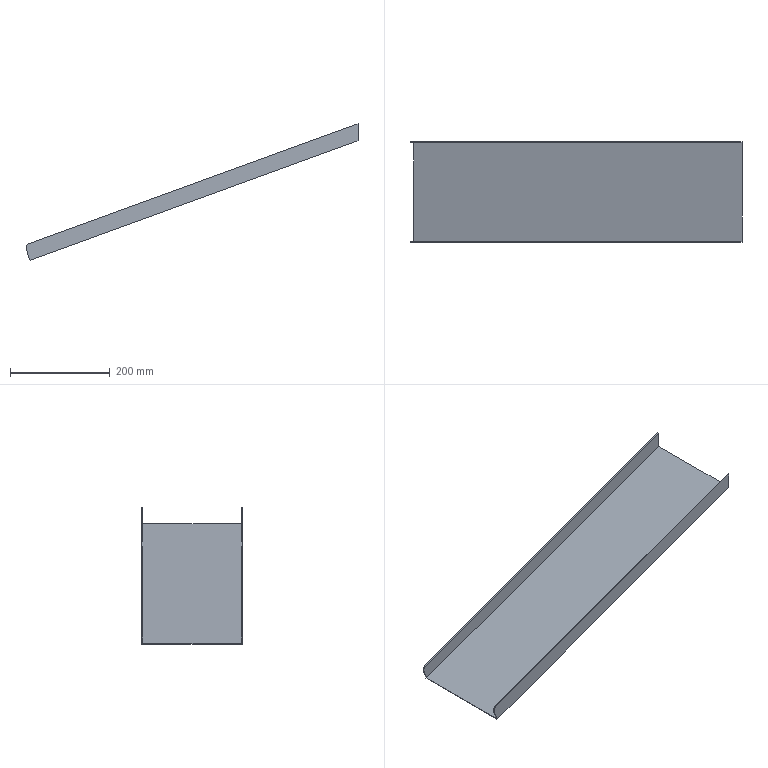Part | NX | features HB 2 | 1 solid | 12 faces | box 664.956 x 201 x 273.12 mm | volume 365672 mm3 | plane 10 | cylinder 2 | commonest cylinder face diameters 20 x2
STEP:
#1=CARTESIAN_POINT('',(3932.421,98.421,-251.344));
#2=VERTEX_POINT('',#1);
#3=CARTESIAN_POINT('',(3274.909,98.421,-490.659));
#4=VERTEX_POINT('',#3);
#5=CARTESIAN_POINT('',(3821.81,98.421,-291.603));
#6=DIRECTION('',(-0.9397,0.,-0.342));
#7=VECTOR('',#6,1000.);
#8=LINE('',#5,#7);
#9=EDGE_CURVE('',#2,#4,#8,.T.);
#10=ORIENTED_EDGE('',*,*,#9,.F.);
#11=CARTESIAN_POINT('',(3932.421,98.421,-219.418));
#12=VERTEX_POINT('',#11);
#13=CARTESIAN_POINT('',(3932.421,98.421,-291.603));
#14=DIRECTION('',(0.,0.,1.));
#15=VECTOR('',#14,1000.);
#16=LINE('',#13,#15);
#17=EDGE_CURVE('',#2,#12,#16,.T.);
#18=ORIENTED_EDGE('',*,*,#17,.T.);
#19=CARTESIAN_POINT('',(3274.045,98.421,-459.048));
#20=VERTEX_POINT('',#19);
#21=CARTESIAN_POINT('',(3811.549,98.421,-263.412));
#22=DIRECTION('',(0.9397,0.,0.342));
#23=VECTOR('',#22,1000.);
#24=LINE('',#21,#23);
#25=EDGE_CURVE('',#20,#12,#24,.T.);
#26=ORIENTED_EDGE('',*,*,#25,.F.);
#27=CARTESIAN_POINT('',(3268.068,98.421,-471.865));
#28=VERTEX_POINT('',#27);
#29=CARTESIAN_POINT('',(3277.465,98.421,-468.445));
#30=DIRECTION('',(0.,1.,0.));
#31=DIRECTION('',(0.,0.,1.));
#32=AXIS2_PLACEMENT_3D('',#29,#30,#31);
#33=CIRCLE('',#32,10.);
#34=EDGE_CURVE('',#28,#20,#33,.T.);
#35=ORIENTED_EDGE('',*,*,#34,.F.);
#36=CARTESIAN_POINT('',(3274.909,98.421,-490.659));
#37=DIRECTION('',(-0.342,0.,0.9397));
#38=VECTOR('',#37,1000.);
#39=LINE('',#36,#38);
#40=EDGE_CURVE('',#4,#28,#39,.T.);
#41=ORIENTED_EDGE('',*,*,#40,.F.);
#42=EDGE_LOOP('',(#10,#18,#26,#35,#41));
#43=FACE_BOUND('',#42,.T.);
#44=CARTESIAN_POINT('',(3821.81,98.421,-291.603));
#45=DIRECTION('',(0.,-1.,0.));
#46=DIRECTION('',(0.08716,0.,0.9962));
#47=AXIS2_PLACEMENT_3D('',#44,#45,#46);
#48=PLANE('',#47);
#49=ADVANCED_FACE('',(#43),#48,.T.);
#50=CARTESIAN_POINT('',(3932.421,-98.579,-219.418));
#51=VERTEX_POINT('',#50);
#52=CARTESIAN_POINT('',(3932.421,-100.579,-219.418));
#53=VERTEX_POINT('',#52);
#54=CARTESIAN_POINT('',(3932.421,-198.579,-219.418));
#55=DIRECTION('',(0.,-1.,0.));
#56=VECTOR('',#55,1000.);
#57=LINE('',#54,#56);
#58=EDGE_CURVE('',#51,#53,#57,.T.);
#59=ORIENTED_EDGE('',*,*,#58,.F.);
#60=CARTESIAN_POINT('',(3274.045,-98.579,-459.048));
#61=VERTEX_POINT('',#60);
#62=CARTESIAN_POINT('',(3811.549,-98.579,-263.412));
#63=DIRECTION('',(0.9397,0.,0.342));
#64=VECTOR('',#63,1000.);
#65=LINE('',#62,#64);
#66=EDGE_CURVE('',#61,#51,#65,.T.);
#67=ORIENTED_EDGE('',*,*,#66,.F.);
#68=CARTESIAN_POINT('',(3274.045,-100.579,-459.048));
#69=VERTEX_POINT('',#68);
#70=CARTESIAN_POINT('',(3274.045,-198.579,-459.048));
#71=DIRECTION('',(0.,1.,0.));
#72=VECTOR('',#71,1000.);
#73=LINE('',#70,#72);
#74=EDGE_CURVE('',#69,#61,#73,.T.);
#75=ORIENTED_EDGE('',*,*,#74,.F.);
#76=CARTESIAN_POINT('',(3811.549,-100.579,-263.412));
#77=DIRECTION('',(0.9397,0.,0.342));
#78=VECTOR('',#77,1000.);
#79=LINE('',#76,#78);
#80=EDGE_CURVE('',#69,#53,#79,.T.);
#81=ORIENTED_EDGE('',*,*,#80,.T.);
#82=EDGE_LOOP('',(#59,#67,#75,#81));
#83=FACE_BOUND('',#82,.T.);
#84=CARTESIAN_POINT('',(3811.549,-198.579,-263.412));
#85=DIRECTION('',(0.342,0.,-0.9397));
#86=DIRECTION('',(-0.9397,0.,-0.342));
#87=AXIS2_PLACEMENT_3D('',#84,#85,#86);
#88=PLANE('',#87);
#89=ADVANCED_FACE('',(#83),#88,.F.);
#90=ORIENTED_EDGE('',*,*,#66,.T.);
#91=CARTESIAN_POINT('',(3932.421,-98.579,-251.344));
#92=VERTEX_POINT('',#91);
#93=CARTESIAN_POINT('',(3932.421,-98.579,-291.603));
#94=DIRECTION('',(0.,0.,-1.));
#95=VECTOR('',#94,1000.);
#96=LINE('',#93,#95);
#97=EDGE_CURVE('',#51,#92,#96,.T.);
#98=ORIENTED_EDGE('',*,*,#97,.T.);
#99=CARTESIAN_POINT('',(3274.909,-98.579,-490.659));
#100=VERTEX_POINT('',#99);
#101=CARTESIAN_POINT('',(3821.81,-98.579,-291.603));
#102=DIRECTION('',(0.9397,0.,0.342));
#103=VECTOR('',#102,1000.);
#104=LINE('',#101,#103);
#105=EDGE_CURVE('',#100,#92,#104,.T.);
#106=ORIENTED_EDGE('',*,*,#105,.F.);
#107=CARTESIAN_POINT('',(3268.068,-98.579,-471.865));
#108=VERTEX_POINT('',#107);
#109=CARTESIAN_POINT('',(3274.909,-98.579,-490.659));
#110=DIRECTION('',(-0.342,0.,0.9397));
#111=VECTOR('',#110,1000.);
#112=LINE('',#109,#111);
#113=EDGE_CURVE('',#100,#108,#112,.T.);
#114=ORIENTED_EDGE('',*,*,#113,.T.);
#115=CARTESIAN_POINT('',(3277.465,-98.579,-468.445));
#116=DIRECTION('',(0.,-1.,0.));
#117=DIRECTION('',(0.08716,0.,0.9962));
#118=AXIS2_PLACEMENT_3D('',#115,#116,#117);
#119=CIRCLE('',#118,10.);
#120=EDGE_CURVE('',#61,#108,#119,.T.);
#121=ORIENTED_EDGE('',*,*,#120,.F.);
#122=EDGE_LOOP('',(#90,#98,#106,#114,#121));
#123=FACE_BOUND('',#122,.T.);
#124=CARTESIAN_POINT('',(3821.81,-98.579,-291.603));
#125=DIRECTION('',(0.,1.,0.));
#126=DIRECTION('',(0.08716,0.,0.9962));
#127=AXIS2_PLACEMENT_3D('',#124,#125,#126);
#128=PLANE('',#127);
#129=ADVANCED_FACE('',(#123),#128,.T.);
#130=CARTESIAN_POINT('',(3932.421,-100.579,-253.472));
#131=VERTEX_POINT('',#130);
#132=CARTESIAN_POINT('',(3932.421,-100.579,-291.603));
#133=DIRECTION('',(0.,0.,-1.));
#134=VECTOR('',#133,1000.);
#135=LINE('',#132,#134);
#136=EDGE_CURVE('',#53,#131,#135,.T.);
#137=ORIENTED_EDGE('',*,*,#136,.F.);
#138=ORIENTED_EDGE('',*,*,#80,.F.);
#139=CARTESIAN_POINT('',(3268.068,-100.579,-471.865));
#140=VERTEX_POINT('',#139);
#141=CARTESIAN_POINT('',(3277.465,-100.579,-468.445));
#142=DIRECTION('',(0.,1.,0.));
#143=DIRECTION('',(0.08716,0.,0.9962));
#144=AXIS2_PLACEMENT_3D('',#141,#142,#143);
#145=CIRCLE('',#144,10.);
#146=EDGE_CURVE('',#140,#69,#145,.T.);
#147=ORIENTED_EDGE('',*,*,#146,.F.);
#148=CARTESIAN_POINT('',(3275.593,-100.579,-492.538));
#149=VERTEX_POINT('',#148);
#150=CARTESIAN_POINT('',(3274.909,-100.579,-490.659));
#151=DIRECTION('',(-0.342,0.,0.9397));
#152=VECTOR('',#151,1000.);
#153=LINE('',#150,#152);
#154=EDGE_CURVE('',#149,#140,#153,.T.);
#155=ORIENTED_EDGE('',*,*,#154,.F.);
#156=CARTESIAN_POINT('',(3822.494,-100.579,-293.482));
#157=DIRECTION('',(-0.9397,0.,-0.342));
#158=VECTOR('',#157,1000.);
#159=LINE('',#156,#158);
#160=EDGE_CURVE('',#131,#149,#159,.T.);
#161=ORIENTED_EDGE('',*,*,#160,.F.);
#162=EDGE_LOOP('',(#137,#138,#147,#155,#161));
#163=FACE_BOUND('',#162,.T.);
#164=CARTESIAN_POINT('',(3821.81,-100.579,-291.603));
#165=DIRECTION('',(0.,1.,0.));
#166=DIRECTION('',(-0.08716,0.,-0.9962));
#167=AXIS2_PLACEMENT_3D('',#164,#165,#166);
#168=PLANE('',#167);
#169=ADVANCED_FACE('',(#163),#168,.F.);
#170=CARTESIAN_POINT('',(3932.421,100.421,-253.472));
#171=VERTEX_POINT('',#170);
#172=CARTESIAN_POINT('',(3932.421,-103.579,-253.472));
#173=DIRECTION('',(0.,1.,0.));
#174=VECTOR('',#173,1000.);
#175=LINE('',#172,#174);
#176=EDGE_CURVE('',#131,#171,#175,.T.);
#177=ORIENTED_EDGE('',*,*,#176,.F.);
#178=ORIENTED_EDGE('',*,*,#160,.T.);
#179=CARTESIAN_POINT('',(3275.593,100.421,-492.538));
#180=VERTEX_POINT('',#179);
#181=CARTESIAN_POINT('',(3275.593,-103.579,-492.538));
#182=DIRECTION('',(0.,1.,0.));
#183=VECTOR('',#182,1000.);
#184=LINE('',#181,#183);
#185=EDGE_CURVE('',#149,#180,#184,.T.);
#186=ORIENTED_EDGE('',*,*,#185,.T.);
#187=CARTESIAN_POINT('',(3822.494,100.421,-293.482));
#188=DIRECTION('',(0.9397,0.,0.342));
#189=VECTOR('',#188,1000.);
#190=LINE('',#187,#189);
#191=EDGE_CURVE('',#180,#171,#190,.T.);
#192=ORIENTED_EDGE('',*,*,#191,.T.);
#193=EDGE_LOOP('',(#177,#178,#186,#192));
#194=FACE_BOUND('',#193,.T.);
#195=CARTESIAN_POINT('',(3822.494,-103.579,-293.482));
#196=DIRECTION('',(-0.342,0.,0.9397));
#197=DIRECTION('',(0.,1.,0.));
#198=AXIS2_PLACEMENT_3D('',#195,#196,#197);
#199=PLANE('',#198);
#200=ADVANCED_FACE('',(#194),#199,.F.);
#201=ORIENTED_EDGE('',*,*,#105,.T.);
#202=CARTESIAN_POINT('',(3932.421,-103.579,-251.344));
#203=DIRECTION('',(0.,1.,0.));
#204=VECTOR('',#203,1000.);
#205=LINE('',#202,#204);
#206=EDGE_CURVE('',#92,#2,#205,.T.);
#207=ORIENTED_EDGE('',*,*,#206,.T.);
#208=ORIENTED_EDGE('',*,*,#9,.T.);
#209=CARTESIAN_POINT('',(3274.909,-103.579,-490.659));
#210=DIRECTION('',(0.,1.,0.));
#211=VECTOR('',#210,1000.);
#212=LINE('',#209,#211);
#213=EDGE_CURVE('',#100,#4,#212,.T.);
#214=ORIENTED_EDGE('',*,*,#213,.F.);
#215=EDGE_LOOP('',(#201,#207,#208,#214));
#216=FACE_BOUND('',#215,.T.);
#217=CARTESIAN_POINT('',(3821.81,-103.579,-291.603));
#218=DIRECTION('',(-0.342,0.,0.9397));
#219=DIRECTION('',(0.,1.,0.));
#220=AXIS2_PLACEMENT_3D('',#217,#218,#219);
#221=PLANE('',#220);
#222=ADVANCED_FACE('',(#216),#221,.T.);
#223=CARTESIAN_POINT('',(3932.421,100.421,-219.418));
#224=VERTEX_POINT('',#223);
#225=CARTESIAN_POINT('',(3932.421,128.421,-219.418));
#226=DIRECTION('',(0.,-1.,0.));
#227=VECTOR('',#226,1000.);
#228=LINE('',#225,#227);
#229=EDGE_CURVE('',#224,#12,#228,.T.);
#230=ORIENTED_EDGE('',*,*,#229,.F.);
#231=CARTESIAN_POINT('',(3274.045,100.421,-459.048));
#232=VERTEX_POINT('',#231);
#233=CARTESIAN_POINT('',(3811.549,100.421,-263.412));
#234=DIRECTION('',(0.9397,0.,0.342));
#235=VECTOR('',#234,1000.);
#236=LINE('',#233,#235);
#237=EDGE_CURVE('',#232,#224,#236,.T.);
#238=ORIENTED_EDGE('',*,*,#237,.F.);
#239=CARTESIAN_POINT('',(3274.045,73.421,-459.048));
#240=DIRECTION('',(0.,1.,0.));
#241=VECTOR('',#240,1000.);
#242=LINE('',#239,#241);
#243=EDGE_CURVE('',#20,#232,#242,.T.);
#244=ORIENTED_EDGE('',*,*,#243,.F.);
#245=ORIENTED_EDGE('',*,*,#25,.T.);
#246=EDGE_LOOP('',(#230,#238,#244,#245));
#247=FACE_BOUND('',#246,.T.);
#248=CARTESIAN_POINT('',(3811.549,128.421,-263.412));
#249=DIRECTION('',(0.342,0.,-0.9397));
#250=DIRECTION('',(-0.9397,0.,-0.342));
#251=AXIS2_PLACEMENT_3D('',#248,#249,#250);
#252=PLANE('',#251);
#253=ADVANCED_FACE('',(#247),#252,.F.);
#254=CARTESIAN_POINT('',(3932.421,100.421,-291.603));
#255=DIRECTION('',(0.,0.,1.));
#256=VECTOR('',#255,1000.);
#257=LINE('',#254,#256);
#258=EDGE_CURVE('',#171,#224,#257,.T.);
#259=ORIENTED_EDGE('',*,*,#258,.F.);
#260=ORIENTED_EDGE('',*,*,#191,.F.);
#261=CARTESIAN_POINT('',(3268.068,100.421,-471.865));
#262=VERTEX_POINT('',#261);
#263=CARTESIAN_POINT('',(3274.909,100.421,-490.659));
#264=DIRECTION('',(-0.342,0.,0.9397));
#265=VECTOR('',#264,1000.);
#266=LINE('',#263,#265);
#267=EDGE_CURVE('',#180,#262,#266,.T.);
#268=ORIENTED_EDGE('',*,*,#267,.T.);
#269=CARTESIAN_POINT('',(3277.465,100.421,-468.445));
#270=DIRECTION('',(0.,-1.,0.));
#271=DIRECTION('',(0.,0.,1.));
#272=AXIS2_PLACEMENT_3D('',#269,#270,#271);
#273=CIRCLE('',#272,10.);
#274=EDGE_CURVE('',#232,#262,#273,.T.);
#275=ORIENTED_EDGE('',*,*,#274,.F.);
#276=ORIENTED_EDGE('',*,*,#237,.T.);
#277=EDGE_LOOP('',(#259,#260,#268,#275,#276));
#278=FACE_BOUND('',#277,.T.);
#279=CARTESIAN_POINT('',(3821.81,100.421,-291.603));
#280=DIRECTION('',(0.,-1.,0.));
#281=DIRECTION('',(0.08716,0.,0.9962));
#282=AXIS2_PLACEMENT_3D('',#279,#280,#281);
#283=PLANE('',#282);
#284=ADVANCED_FACE('',(#278),#283,.F.);
#285=ORIENTED_EDGE('',*,*,#120,.T.);
#286=CARTESIAN_POINT('',(3268.068,-198.579,-471.865));
#287=DIRECTION('',(0.,-1.,0.));
#288=VECTOR('',#287,1000.);
#289=LINE('',#286,#288);
#290=EDGE_CURVE('',#108,#140,#289,.T.);
#291=ORIENTED_EDGE('',*,*,#290,.T.);
#292=ORIENTED_EDGE('',*,*,#146,.T.);
#293=ORIENTED_EDGE('',*,*,#74,.T.);
#294=EDGE_LOOP('',(#285,#291,#292,#293));
#295=FACE_BOUND('',#294,.T.);
#296=CARTESIAN_POINT('',(3277.465,-198.579,-468.445));
#297=DIRECTION('',(0.,-1.,0.));
#298=DIRECTION('',(0.08716,0.,0.9962));
#299=AXIS2_PLACEMENT_3D('',#296,#297,#298);
#300=CYLINDRICAL_SURFACE('',#299,10.);
#301=ADVANCED_FACE('',(#295),#300,.T.);
#302=ORIENTED_EDGE('',*,*,#213,.T.);
#303=ORIENTED_EDGE('',*,*,#40,.T.);
#304=CARTESIAN_POINT('',(3268.068,-184.579,-471.865));
#305=DIRECTION('',(0.,-1.,0.));
#306=VECTOR('',#305,1000.);
#307=LINE('',#304,#306);
#308=EDGE_CURVE('',#262,#28,#307,.T.);
#309=ORIENTED_EDGE('',*,*,#308,.F.);
#310=ORIENTED_EDGE('',*,*,#267,.F.);
#311=ORIENTED_EDGE('',*,*,#185,.F.);
#312=ORIENTED_EDGE('',*,*,#154,.T.);
#313=ORIENTED_EDGE('',*,*,#290,.F.);
#314=ORIENTED_EDGE('',*,*,#113,.F.);
#315=EDGE_LOOP('',(#302,#303,#309,#310,#311,#312,#313,#314));
#316=FACE_BOUND('',#315,.T.);
#317=CARTESIAN_POINT('',(3274.909,-103.579,-490.659));
#318=DIRECTION('',(0.9397,0.,0.342));
#319=DIRECTION('',(0.342,0.,-0.9397));
#320=AXIS2_PLACEMENT_3D('',#317,#318,#319);
#321=PLANE('',#320);
#322=ADVANCED_FACE('',(#316),#321,.F.);
#323=ORIENTED_EDGE('',*,*,#34,.T.);
#324=ORIENTED_EDGE('',*,*,#243,.T.);
#325=ORIENTED_EDGE('',*,*,#274,.T.);
#326=ORIENTED_EDGE('',*,*,#308,.T.);
#327=EDGE_LOOP('',(#323,#324,#325,#326));
#328=FACE_BOUND('',#327,.T.);
#329=CARTESIAN_POINT('',(3277.465,-184.579,-468.445));
#330=DIRECTION('',(0.,1.,0.));
#331=DIRECTION('',(-0.08716,0.,-0.9962));
#332=AXIS2_PLACEMENT_3D('',#329,#330,#331);
#333=CYLINDRICAL_SURFACE('',#332,10.);
#334=ADVANCED_FACE('',(#328),#333,.T.);
#335=ORIENTED_EDGE('',*,*,#97,.F.);
#336=ORIENTED_EDGE('',*,*,#58,.T.);
#337=ORIENTED_EDGE('',*,*,#136,.T.);
#338=ORIENTED_EDGE('',*,*,#176,.T.);
#339=ORIENTED_EDGE('',*,*,#258,.T.);
#340=ORIENTED_EDGE('',*,*,#229,.T.);
#341=ORIENTED_EDGE('',*,*,#17,.F.);
#342=ORIENTED_EDGE('',*,*,#206,.F.);
#343=EDGE_LOOP('',(#335,#336,#337,#338,#339,#340,#341,#342));
#344=FACE_BOUND('',#343,.T.);
#345=CARTESIAN_POINT('',(3932.421,520.421,85.));
#346=DIRECTION('',(1.,0.,0.));
#347=DIRECTION('',(0.,0.,1.));
#348=AXIS2_PLACEMENT_3D('',#345,#346,#347);
#349=PLANE('',#348);
#350=ADVANCED_FACE('',(#344),#349,.T.);
#351=CLOSED_SHELL('',(#49,#89,#129,#169,#200,#222,#253,#284,#301,#322,#334,#350));
#352=MANIFOLD_SOLID_BREP('',#351);
#353=(LENGTH_UNIT()NAMED_UNIT(*)SI_UNIT(.MILLI.,.METRE.));
#354=UNCERTAINTY_MEASURE_WITH_UNIT(LENGTH_MEASURE(0.00001),#353,'','');
#355=(NAMED_UNIT(*)PLANE_ANGLE_UNIT()SI_UNIT($,.RADIAN.));
#356=(NAMED_UNIT(*)SI_UNIT($,.STERADIAN.)SOLID_ANGLE_UNIT());
#357=(GEOMETRIC_REPRESENTATION_CONTEXT(3)GLOBAL_UNCERTAINTY_ASSIGNED_CONTEXT((#354))GLOBAL_UNIT_ASSIGNED_CONTEXT((#353,#355,#356))REPRESENTATION_CONTEXT('',''));
#358=ADVANCED_BREP_SHAPE_REPRESENTATION('',(#352),#357);